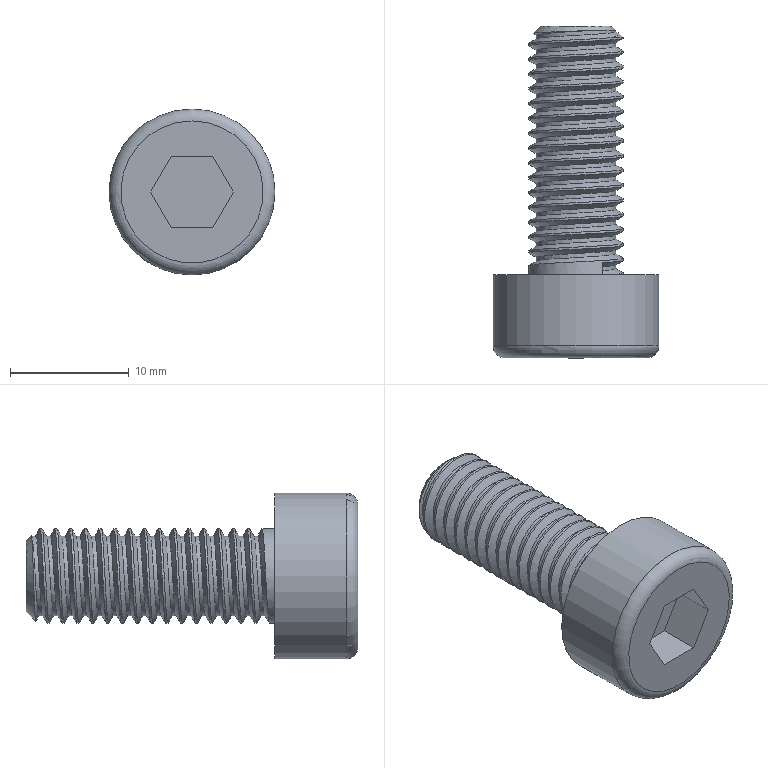Part | NX | features DATUM_CSYS 3, EXTRUDE 3, DATUM_PLANE 2, SKETCH 2, BLEND 1, CHAMFER 1, THREADS 1 | 1 solid | 20 faces | box 14 x 28 x 14 mm | volume 1799 mm3 | plane 11 | cylinder 3 | spline 3 | cone 2 | torus 1 | commonest cylinder face diameters 6.75 x1 8 x1 14 x1